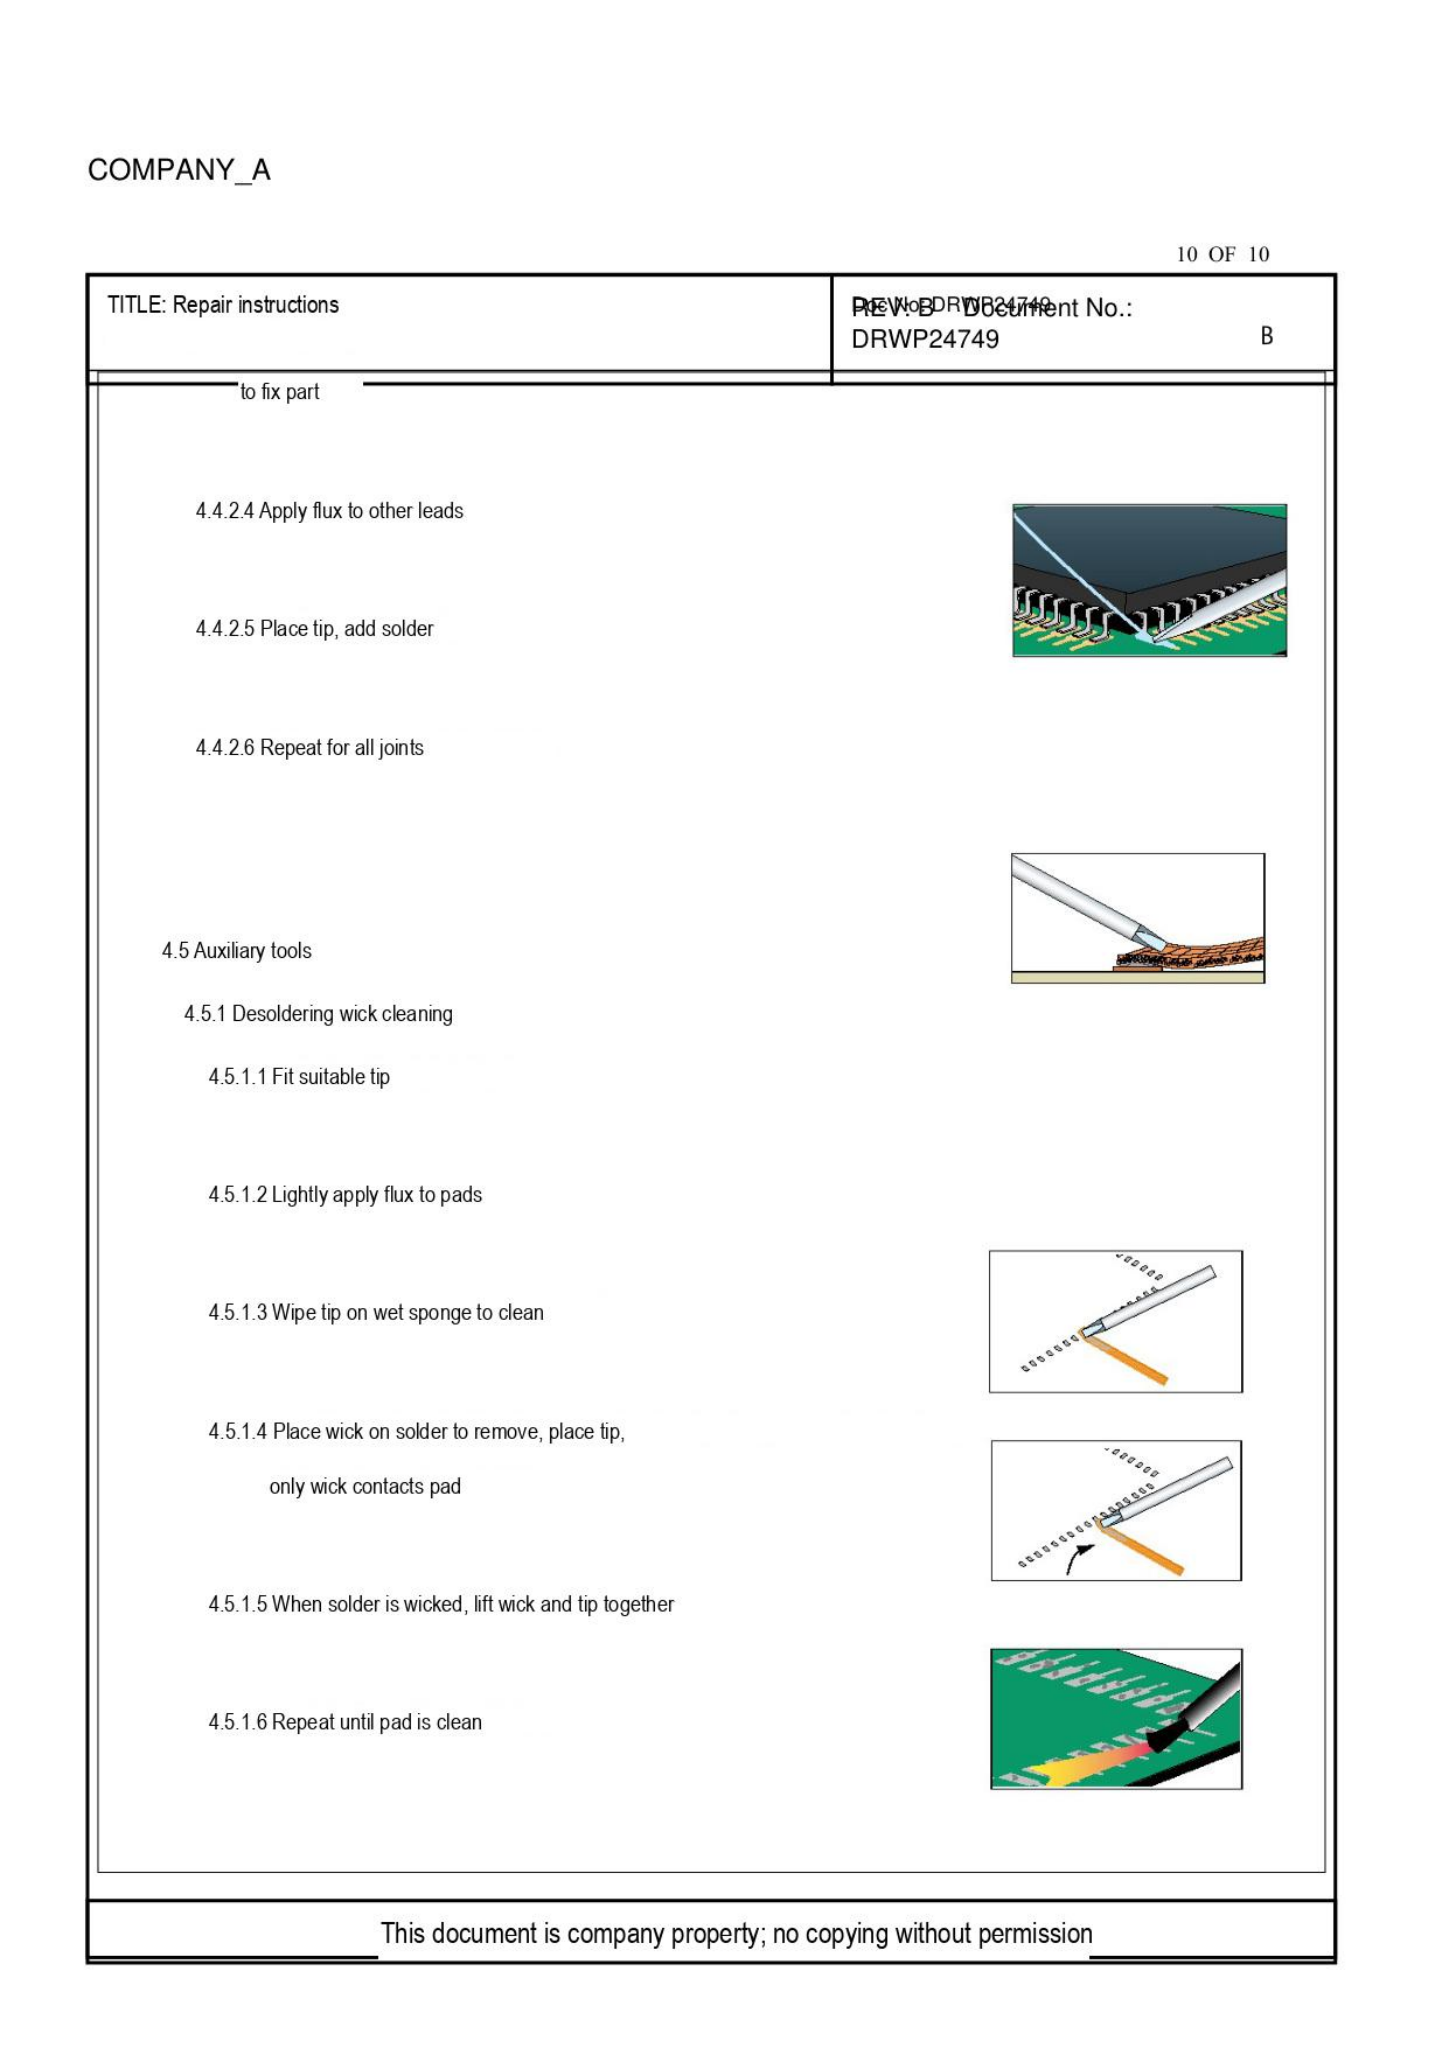COMPANY_A

10 OF 10

| TITLE: Repair instructions | REV: B Document No.: DRWP24749 B |
|---|---|

to fix part

4.4.2.4 Apply flux to other leads

4.4.2.5 Place tip, add solder

4.4.2.6 Repeat for all joints

4.5 Auxiliary tools

4.5.1 Desoldering wick cleaning

4.5.1.1 Fit suitable tip

4.5.1.2 Lightly apply flux to pads

4.5.1.3 Wipe tip on wet sponge to clean

4.5.1.4 Place wick on solder to remove, place tip,

only wick contacts pad

4.5.1.5 When solder is wicked, lift wick and tip together

4.5.1.6 Repeat until pad is clean

This document is company property; no copying without permission
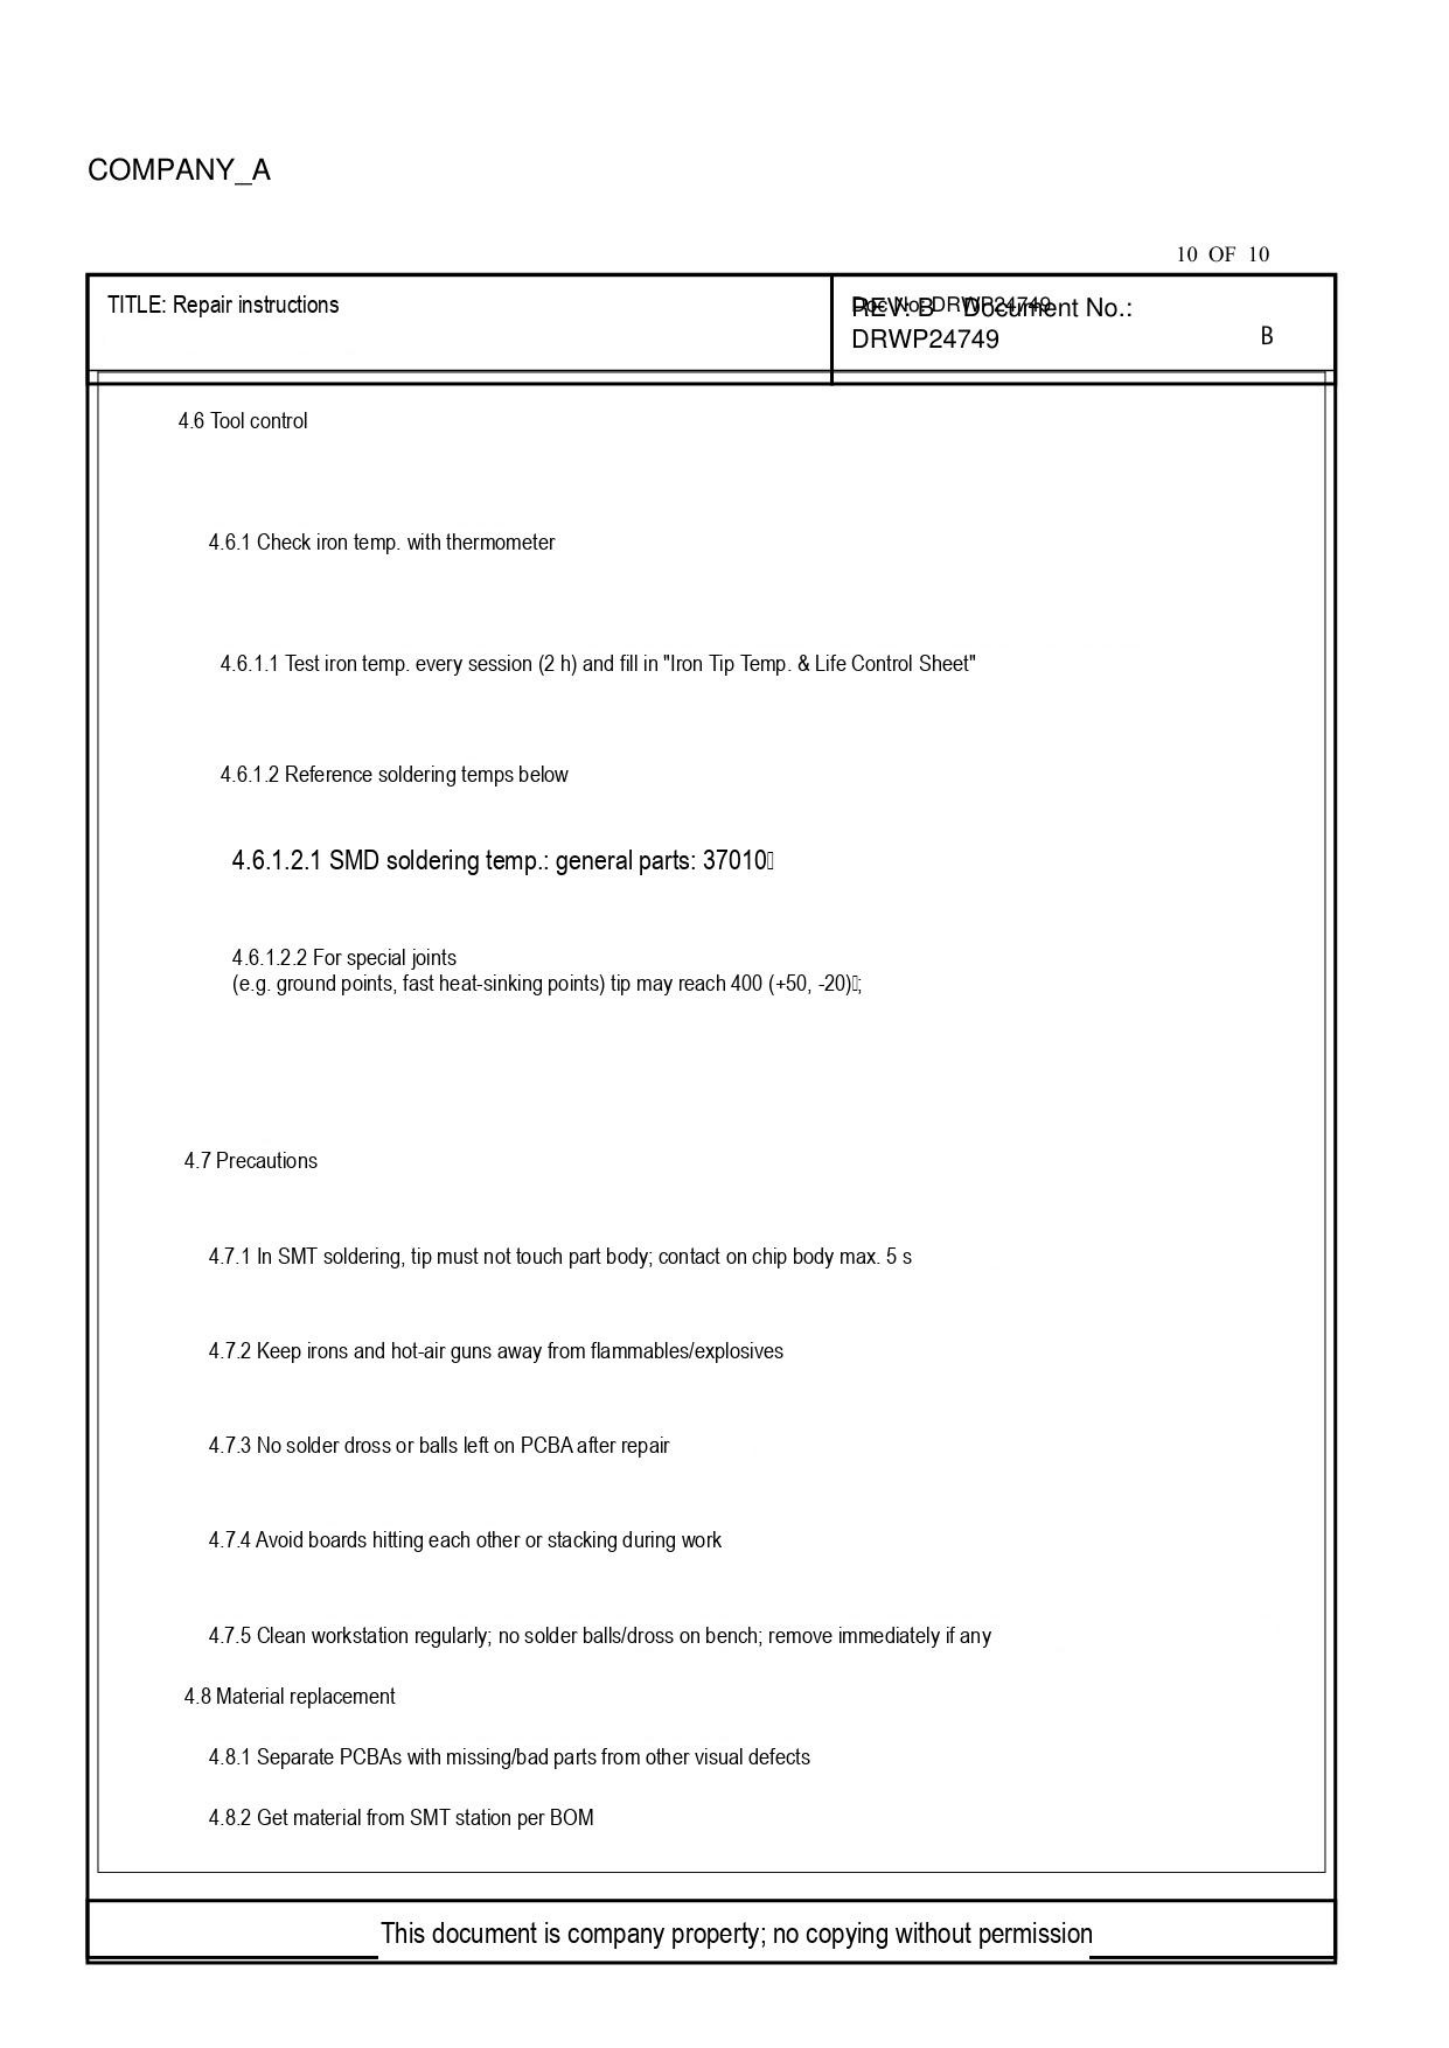COMPANY_A

10 OF 10

| TITLE: Repair instructions | REV: B Document No.: DRWP24749 B |
|---|---|

4.6 Tool control

4.6.1 Check iron temp. with thermometer

4.6.1.1 Test iron temp. every session (2 h) and fill in "Iron Tip Temp. & Life Control Sheet"

4.6.1.2 Reference soldering temps below

4.6.1.2.1 SMD soldering temp.: general parts: 37010

4.6.1.2.2 For special joints
(e.g. ground points, fast heat-sinking points) tip may reach 400 (+50, -20);

4.7 Precautions

4.7.1 In SMT soldering, tip must not touch part body; contact on chip body max. 5 s

4.7.2 Keep irons and hot-air guns away from flammables/explosives

4.7.3 No solder dross or balls left on PCBA after repair

4.7.4 Avoid boards hitting each other or stacking during work

4.7.5 Clean workstation regularly; no solder balls/dross on bench; remove immediately if any

4.8 Material replacement

4.8.1 Separate PCBAs with missing/bad parts from other visual defects

4.8.2 Get material from SMT station per BOM

This document is company property; no copying without permission
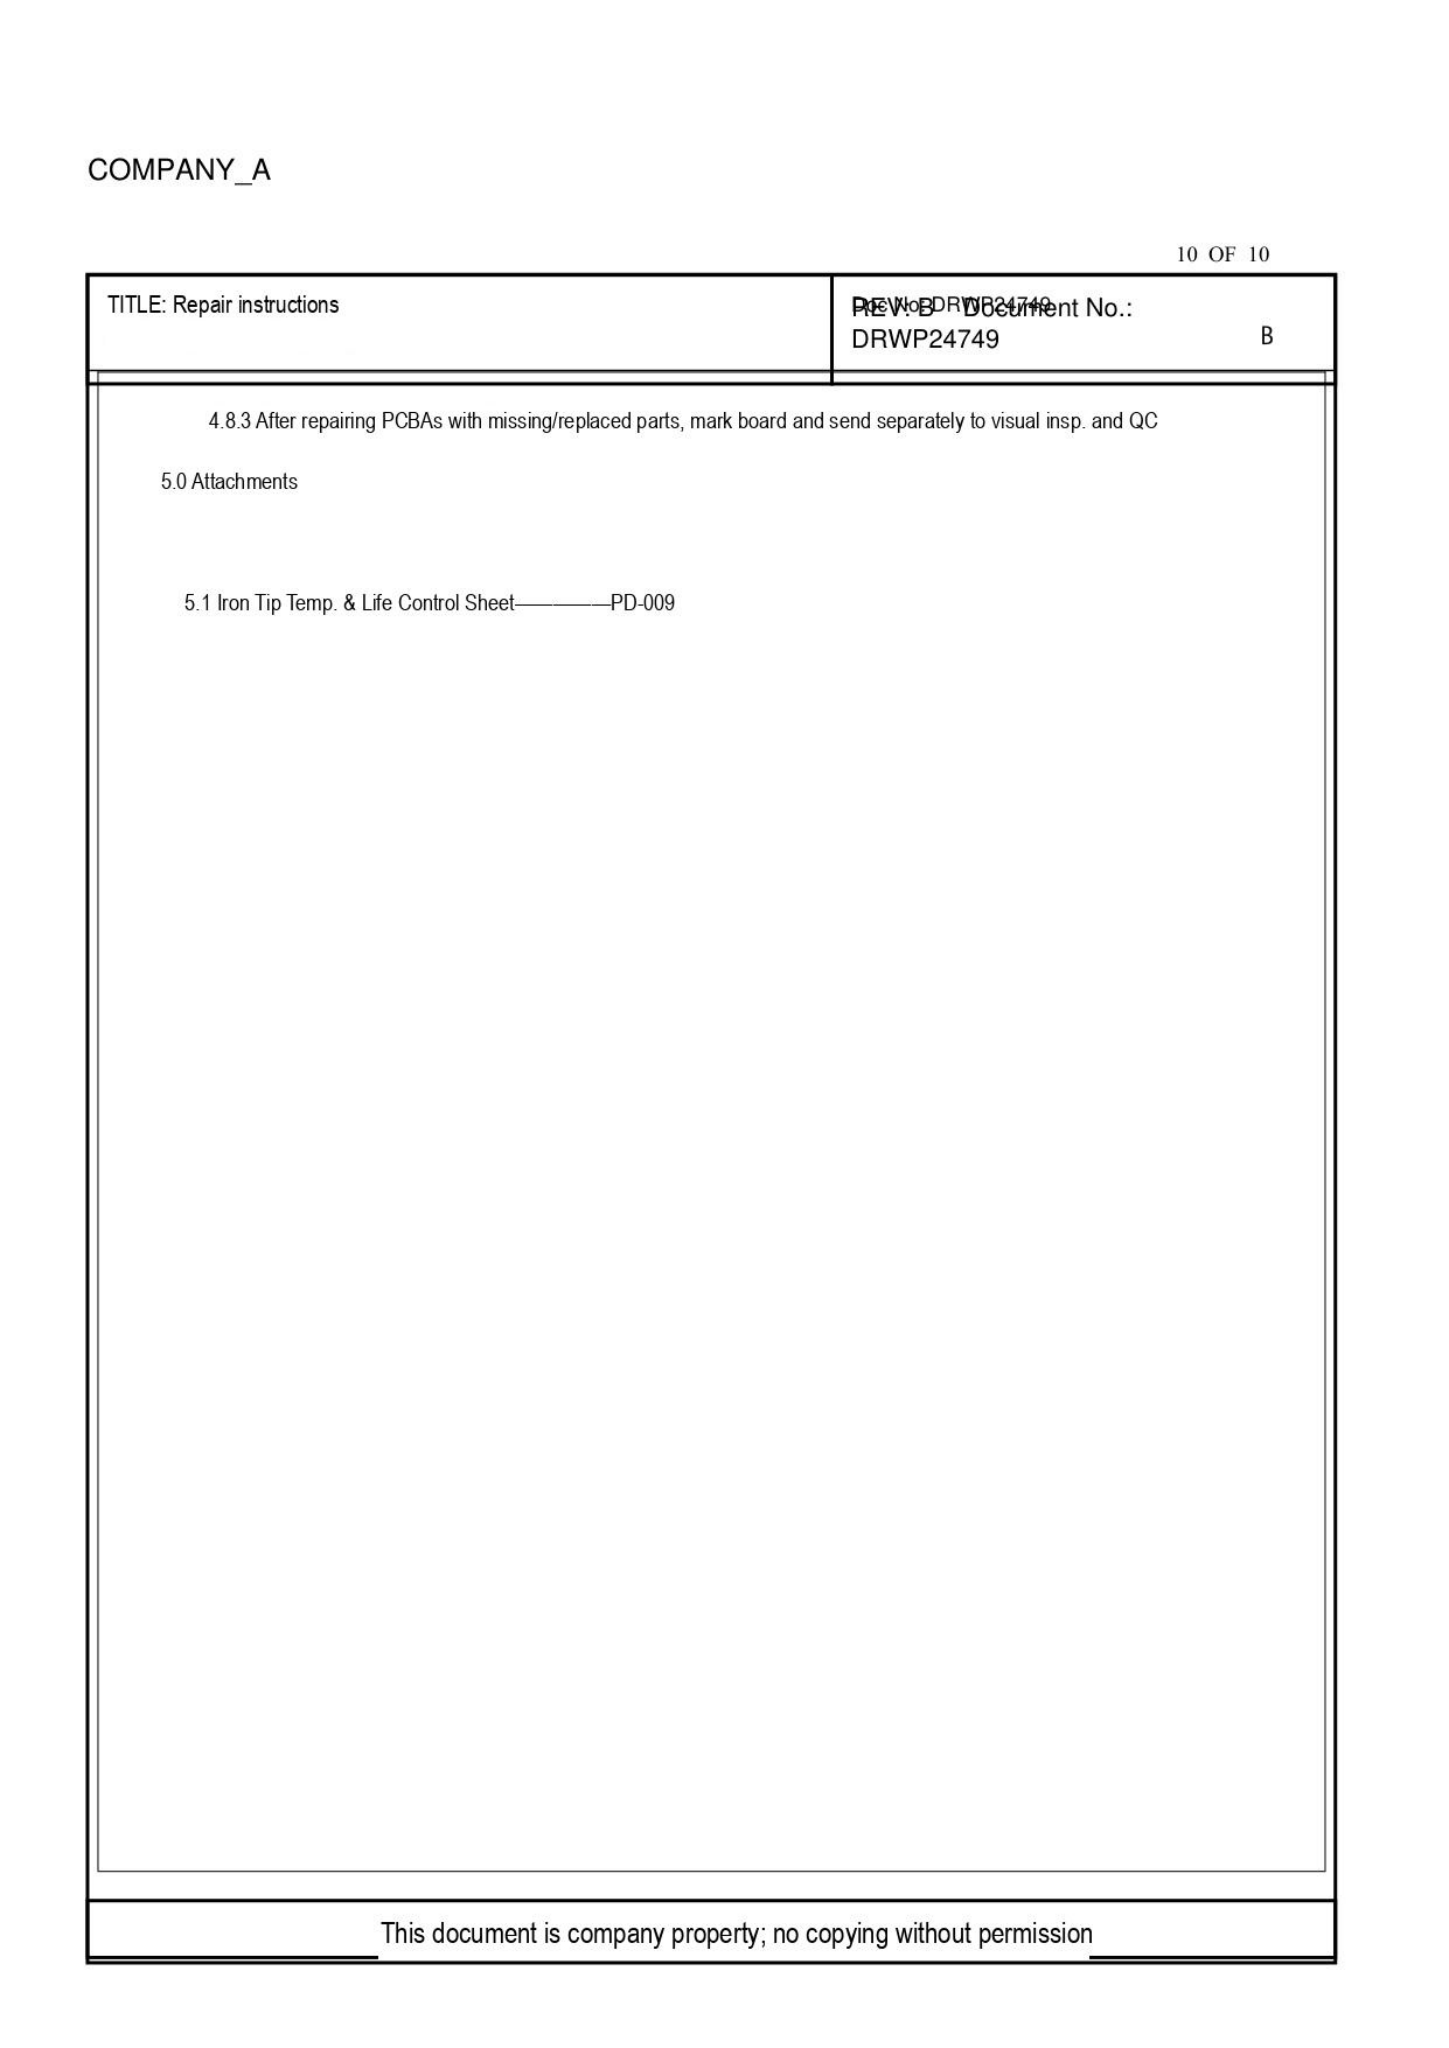COMPANY_A

10 OF 10

| TITLE: Repair instructions | REV: B Document No.: DRWP24749 B |
|---|---|

4.8.3 After repairing PCBAs with missing/replaced parts, mark board and send separately to visual insp. and QC

5.0 Attachments

5.1 Iron Tip Temp. & Life Control Sheet—————PD-009

This document is company property; no copying without permission
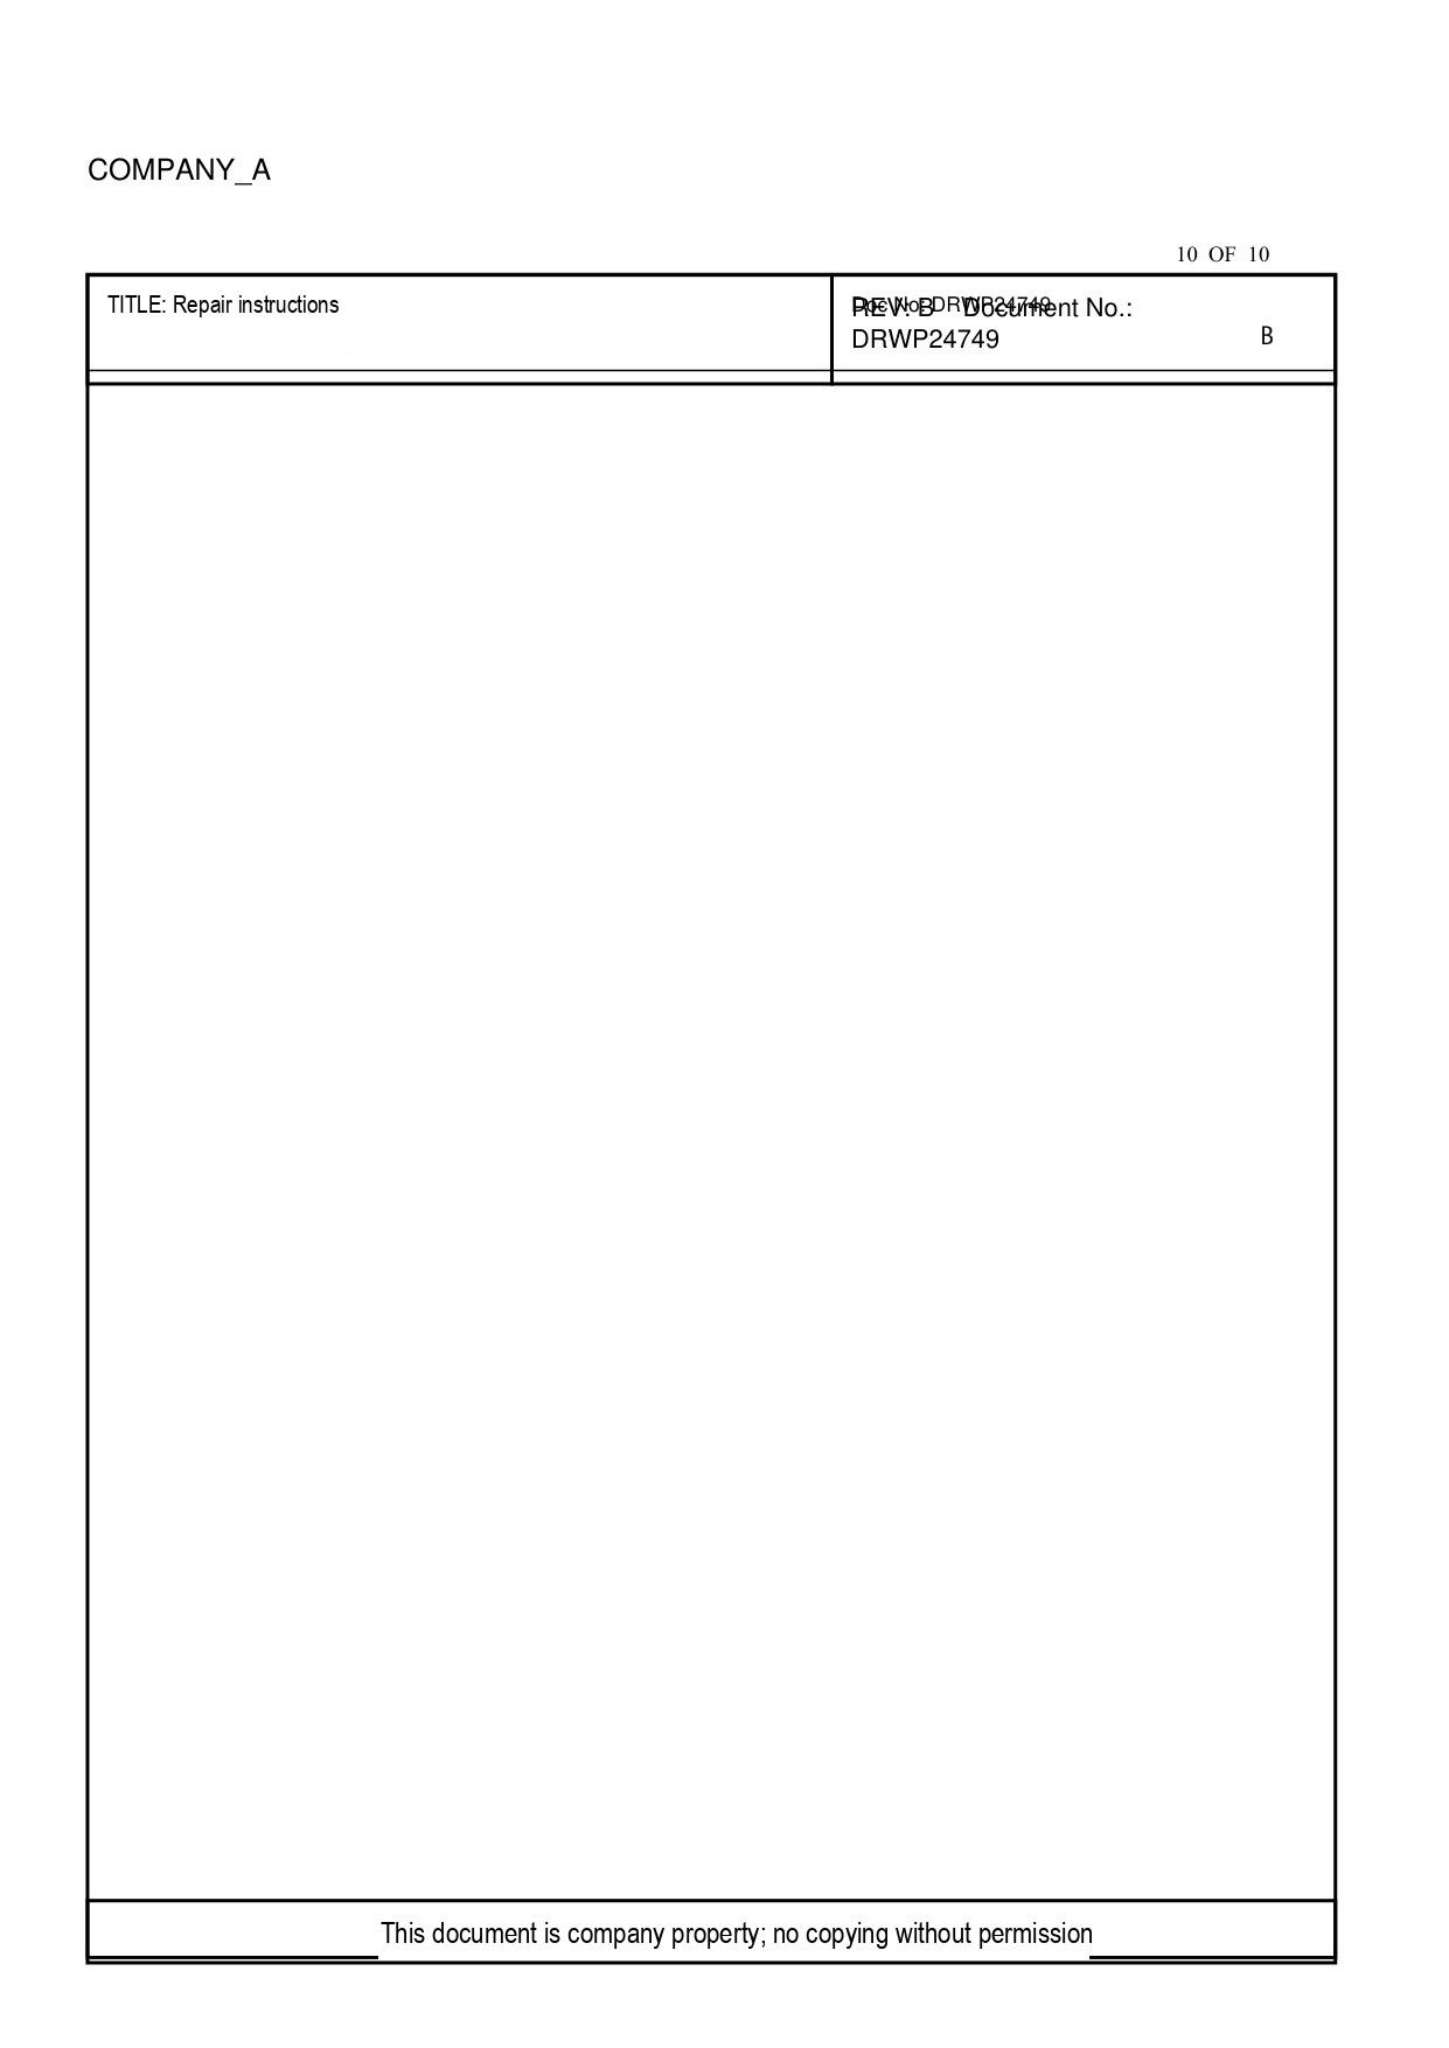COMPANY_A

10 OF 10

| TITLE: Repair instructions | REV: B Document No.: DRWP24749 B |
|---|---|

This document is company property; no copying without permission